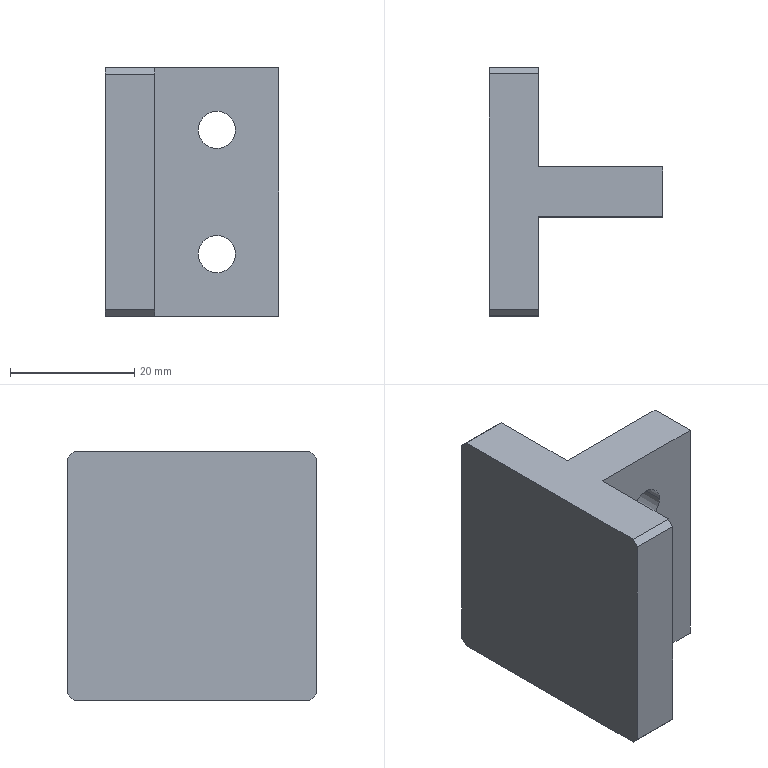Part | SolidWorks | features ICE 2, Chamfer 1, Extrusion 1 | 1 solid | 18 faces | box 28 x 40 x 40 mm | volume 18732 mm3 | plane 14 | cylinder 4 | commonest cylinder face diameters 6 x4
STEP:
#1=CARTESIAN_POINT('',(15.,16.,30.));
#2=VERTEX_POINT('',#1);
#3=CARTESIAN_POINT('',(21.,16.,30.));
#4=VERTEX_POINT('',#3);
#5=CARTESIAN_POINT('',(18.,16.,30.));
#6=DIRECTION('',(0.,-1.,0.));
#7=DIRECTION('',(1.,0.,0.));
#8=AXIS2_PLACEMENT_3D('',#5,#6,#7);
#9=CIRCLE('',#8,3.);
#10=EDGE_CURVE('',#2,#4,#9,.T.);
#11=ORIENTED_EDGE('',*,*,#10,.T.);
#12=CARTESIAN_POINT('',(21.,24.,30.));
#13=VERTEX_POINT('',#12);
#14=CARTESIAN_POINT('',(21.,0.,30.));
#15=DIRECTION('',(0.,1.,0.));
#16=VECTOR('',#15,1000.);
#17=LINE('',#14,#16);
#18=EDGE_CURVE('',#4,#13,#17,.T.);
#19=ORIENTED_EDGE('',*,*,#18,.T.);
#20=CARTESIAN_POINT('',(15.,24.,30.));
#21=VERTEX_POINT('',#20);
#22=CARTESIAN_POINT('',(18.,24.,30.));
#23=DIRECTION('',(0.,1.,0.));
#24=DIRECTION('',(-1.,0.,0.));
#25=AXIS2_PLACEMENT_3D('',#22,#23,#24);
#26=CIRCLE('',#25,3.);
#27=EDGE_CURVE('',#13,#21,#26,.T.);
#28=ORIENTED_EDGE('',*,*,#27,.T.);
#29=CARTESIAN_POINT('',(15.,0.,30.));
#30=DIRECTION('',(0.,1.,0.));
#31=VECTOR('',#30,1000.);
#32=LINE('',#29,#31);
#33=EDGE_CURVE('',#2,#21,#32,.T.);
#34=ORIENTED_EDGE('',*,*,#33,.F.);
#35=EDGE_LOOP('',(#11,#19,#28,#34));
#36=FACE_OUTER_BOUND('',#35,.T.);
#37=CARTESIAN_POINT('',(18.,0.,30.));
#38=DIRECTION('',(0.,1.,0.));
#39=DIRECTION('',(-1.,0.,0.));
#40=AXIS2_PLACEMENT_3D('',#37,#38,#39);
#41=CYLINDRICAL_SURFACE('',#40,3.);
#42=ADVANCED_FACE('',(#36),#41,.F.);
#43=CARTESIAN_POINT('',(15.,16.,10.));
#44=VERTEX_POINT('',#43);
#45=CARTESIAN_POINT('',(21.,16.,10.));
#46=VERTEX_POINT('',#45);
#47=CARTESIAN_POINT('',(18.,16.,10.));
#48=DIRECTION('',(0.,-1.,0.));
#49=DIRECTION('',(1.,0.,0.));
#50=AXIS2_PLACEMENT_3D('',#47,#48,#49);
#51=CIRCLE('',#50,3.);
#52=EDGE_CURVE('',#44,#46,#51,.T.);
#53=ORIENTED_EDGE('',*,*,#52,.T.);
#54=CARTESIAN_POINT('',(21.,24.,10.));
#55=VERTEX_POINT('',#54);
#56=CARTESIAN_POINT('',(21.,0.,10.));
#57=DIRECTION('',(0.,1.,0.));
#58=VECTOR('',#57,1000.);
#59=LINE('',#56,#58);
#60=EDGE_CURVE('',#46,#55,#59,.T.);
#61=ORIENTED_EDGE('',*,*,#60,.T.);
#62=CARTESIAN_POINT('',(15.,24.,10.));
#63=VERTEX_POINT('',#62);
#64=CARTESIAN_POINT('',(18.,24.,10.));
#65=DIRECTION('',(0.,1.,0.));
#66=DIRECTION('',(-1.,0.,0.));
#67=AXIS2_PLACEMENT_3D('',#64,#65,#66);
#68=CIRCLE('',#67,3.);
#69=EDGE_CURVE('',#55,#63,#68,.T.);
#70=ORIENTED_EDGE('',*,*,#69,.T.);
#71=CARTESIAN_POINT('',(15.,0.,10.));
#72=DIRECTION('',(0.,1.,0.));
#73=VECTOR('',#72,1000.);
#74=LINE('',#71,#73);
#75=EDGE_CURVE('',#44,#63,#74,.T.);
#76=ORIENTED_EDGE('',*,*,#75,.F.);
#77=EDGE_LOOP('',(#53,#61,#70,#76));
#78=FACE_OUTER_BOUND('',#77,.T.);
#79=CARTESIAN_POINT('',(18.,0.,10.));
#80=DIRECTION('',(0.,1.,0.));
#81=DIRECTION('',(-1.,0.,0.));
#82=AXIS2_PLACEMENT_3D('',#79,#80,#81);
#83=CYLINDRICAL_SURFACE('',#82,3.);
#84=ADVANCED_FACE('',(#78),#83,.F.);
#85=CARTESIAN_POINT('',(8.,24.,0.));
#86=VERTEX_POINT('',#85);
#87=CARTESIAN_POINT('',(8.,24.,40.));
#88=VERTEX_POINT('',#87);
#89=CARTESIAN_POINT('',(8.,24.,0.));
#90=DIRECTION('',(0.,0.,1.));
#91=VECTOR('',#90,1000.);
#92=LINE('',#89,#91);
#93=EDGE_CURVE('',#86,#88,#92,.T.);
#94=ORIENTED_EDGE('',*,*,#93,.F.);
#95=CARTESIAN_POINT('',(8.,39.,0.));
#96=VERTEX_POINT('',#95);
#97=CARTESIAN_POINT('',(8.,40.,0.));
#98=DIRECTION('',(0.,-1.,0.));
#99=VECTOR('',#98,1000.);
#100=LINE('',#97,#99);
#101=EDGE_CURVE('',#96,#86,#100,.T.);
#102=ORIENTED_EDGE('',*,*,#101,.F.);
#103=CARTESIAN_POINT('',(8.,40.,1.));
#104=VERTEX_POINT('',#103);
#105=CARTESIAN_POINT('',(8.,40.,1.));
#106=DIRECTION('',(0.,0.7071,0.7071));
#107=VECTOR('',#106,1000.);
#108=LINE('',#105,#107);
#109=EDGE_CURVE('',#96,#104,#108,.T.);
#110=ORIENTED_EDGE('',*,*,#109,.T.);
#111=CARTESIAN_POINT('',(8.,40.,39.));
#112=VERTEX_POINT('',#111);
#113=CARTESIAN_POINT('',(8.,40.,0.));
#114=DIRECTION('',(0.,0.,-1.));
#115=VECTOR('',#114,1000.);
#116=LINE('',#113,#115);
#117=EDGE_CURVE('',#112,#104,#116,.T.);
#118=ORIENTED_EDGE('',*,*,#117,.F.);
#119=CARTESIAN_POINT('',(8.,39.,40.));
#120=VERTEX_POINT('',#119);
#121=CARTESIAN_POINT('',(8.,40.,39.));
#122=DIRECTION('',(0.,-0.7071,0.7071));
#123=VECTOR('',#122,1000.);
#124=LINE('',#121,#123);
#125=EDGE_CURVE('',#112,#120,#124,.T.);
#126=ORIENTED_EDGE('',*,*,#125,.T.);
#127=CARTESIAN_POINT('',(8.,40.,40.));
#128=DIRECTION('',(0.,-1.,0.));
#129=VECTOR('',#128,1000.);
#130=LINE('',#127,#129);
#131=EDGE_CURVE('',#120,#88,#130,.T.);
#132=ORIENTED_EDGE('',*,*,#131,.T.);
#133=EDGE_LOOP('',(#94,#102,#110,#118,#126,#132));
#134=FACE_OUTER_BOUND('',#133,.T.);
#135=CARTESIAN_POINT('',(8.,40.,0.));
#136=DIRECTION('',(-1.,0.,0.));
#137=DIRECTION('',(0.,0.,1.));
#138=AXIS2_PLACEMENT_3D('',#135,#136,#137);
#139=PLANE('',#138);
#140=ADVANCED_FACE('',(#134),#139,.F.);
#141=CARTESIAN_POINT('',(0.,39.,40.));
#142=VERTEX_POINT('',#141);
#143=CARTESIAN_POINT('',(0.,1.,40.));
#144=VERTEX_POINT('',#143);
#145=CARTESIAN_POINT('',(0.,40.,40.));
#146=DIRECTION('',(0.,-1.,0.));
#147=VECTOR('',#146,1000.);
#148=LINE('',#145,#147);
#149=EDGE_CURVE('',#142,#144,#148,.T.);
#150=ORIENTED_EDGE('',*,*,#149,.F.);
#151=CARTESIAN_POINT('',(0.,40.,39.));
#152=VERTEX_POINT('',#151);
#153=CARTESIAN_POINT('',(0.,40.,39.));
#154=DIRECTION('',(0.,0.7071,-0.7071));
#155=VECTOR('',#154,1000.);
#156=LINE('',#153,#155);
#157=EDGE_CURVE('',#142,#152,#156,.T.);
#158=ORIENTED_EDGE('',*,*,#157,.T.);
#159=CARTESIAN_POINT('',(0.,40.,1.));
#160=VERTEX_POINT('',#159);
#161=CARTESIAN_POINT('',(0.,40.,0.));
#162=DIRECTION('',(0.,0.,1.));
#163=VECTOR('',#162,1000.);
#164=LINE('',#161,#163);
#165=EDGE_CURVE('',#160,#152,#164,.T.);
#166=ORIENTED_EDGE('',*,*,#165,.F.);
#167=CARTESIAN_POINT('',(0.,39.,0.));
#168=VERTEX_POINT('',#167);
#169=CARTESIAN_POINT('',(0.,40.,1.));
#170=DIRECTION('',(0.,-0.7071,-0.7071));
#171=VECTOR('',#170,1000.);
#172=LINE('',#169,#171);
#173=EDGE_CURVE('',#160,#168,#172,.T.);
#174=ORIENTED_EDGE('',*,*,#173,.T.);
#175=CARTESIAN_POINT('',(0.,1.,0.));
#176=VERTEX_POINT('',#175);
#177=CARTESIAN_POINT('',(0.,40.,0.));
#178=DIRECTION('',(0.,-1.,0.));
#179=VECTOR('',#178,1000.);
#180=LINE('',#177,#179);
#181=EDGE_CURVE('',#168,#176,#180,.T.);
#182=ORIENTED_EDGE('',*,*,#181,.T.);
#183=CARTESIAN_POINT('',(0.,0.,1.));
#184=VERTEX_POINT('',#183);
#185=CARTESIAN_POINT('',(0.,1.,0.));
#186=DIRECTION('',(0.,-0.7071,0.7071));
#187=VECTOR('',#186,1000.);
#188=LINE('',#185,#187);
#189=EDGE_CURVE('',#176,#184,#188,.T.);
#190=ORIENTED_EDGE('',*,*,#189,.T.);
#191=CARTESIAN_POINT('',(0.,0.,39.));
#192=VERTEX_POINT('',#191);
#193=CARTESIAN_POINT('',(0.,0.,0.));
#194=DIRECTION('',(0.,0.,1.));
#195=VECTOR('',#194,1000.);
#196=LINE('',#193,#195);
#197=EDGE_CURVE('',#184,#192,#196,.T.);
#198=ORIENTED_EDGE('',*,*,#197,.T.);
#199=CARTESIAN_POINT('',(0.,1.,40.));
#200=DIRECTION('',(0.,0.7071,0.7071));
#201=VECTOR('',#200,1000.);
#202=LINE('',#199,#201);
#203=EDGE_CURVE('',#192,#144,#202,.T.);
#204=ORIENTED_EDGE('',*,*,#203,.T.);
#205=EDGE_LOOP('',(#150,#158,#166,#174,#182,#190,#198,#204));
#206=FACE_OUTER_BOUND('',#205,.T.);
#207=CARTESIAN_POINT('',(0.,40.,0.));
#208=DIRECTION('',(1.,0.,0.));
#209=DIRECTION('',(0.,0.,-1.));
#210=AXIS2_PLACEMENT_3D('',#207,#208,#209);
#211=PLANE('',#210);
#212=ADVANCED_FACE('',(#206),#211,.F.);
#213=ORIENTED_EDGE('',*,*,#131,.F.);
#214=CARTESIAN_POINT('',(0.,39.,40.));
#215=DIRECTION('',(-1.,0.,0.));
#216=VECTOR('',#215,1000.);
#217=LINE('',#214,#216);
#218=EDGE_CURVE('',#120,#142,#217,.T.);
#219=ORIENTED_EDGE('',*,*,#218,.T.);
#220=ORIENTED_EDGE('',*,*,#149,.T.);
#221=CARTESIAN_POINT('',(8.,1.,40.));
#222=VERTEX_POINT('',#221);
#223=CARTESIAN_POINT('',(0.,1.,40.));
#224=DIRECTION('',(1.,0.,0.));
#225=VECTOR('',#224,1000.);
#226=LINE('',#223,#225);
#227=EDGE_CURVE('',#144,#222,#226,.T.);
#228=ORIENTED_EDGE('',*,*,#227,.T.);
#229=CARTESIAN_POINT('',(8.,16.,40.));
#230=VERTEX_POINT('',#229);
#231=CARTESIAN_POINT('',(8.,40.,40.));
#232=DIRECTION('',(0.,-1.,0.));
#233=VECTOR('',#232,1000.);
#234=LINE('',#231,#233);
#235=EDGE_CURVE('',#230,#222,#234,.T.);
#236=ORIENTED_EDGE('',*,*,#235,.F.);
#237=CARTESIAN_POINT('',(28.,16.,40.));
#238=VERTEX_POINT('',#237);
#239=CARTESIAN_POINT('',(28.,16.,40.));
#240=DIRECTION('',(1.,0.,0.));
#241=VECTOR('',#240,1000.);
#242=LINE('',#239,#241);
#243=EDGE_CURVE('',#230,#238,#242,.T.);
#244=ORIENTED_EDGE('',*,*,#243,.T.);
#245=CARTESIAN_POINT('',(28.,24.,40.));
#246=VERTEX_POINT('',#245);
#247=CARTESIAN_POINT('',(28.,24.,40.));
#248=DIRECTION('',(0.,1.,0.));
#249=VECTOR('',#248,1000.);
#250=LINE('',#247,#249);
#251=EDGE_CURVE('',#238,#246,#250,.T.);
#252=ORIENTED_EDGE('',*,*,#251,.T.);
#253=CARTESIAN_POINT('',(28.,24.,40.));
#254=DIRECTION('',(-1.,0.,0.));
#255=VECTOR('',#254,1000.);
#256=LINE('',#253,#255);
#257=EDGE_CURVE('',#246,#88,#256,.T.);
#258=ORIENTED_EDGE('',*,*,#257,.T.);
#259=EDGE_LOOP('',(#213,#219,#220,#228,#236,#244,#252,#258));
#260=FACE_OUTER_BOUND('',#259,.T.);
#261=CARTESIAN_POINT('',(0.,40.,40.));
#262=DIRECTION('',(0.,0.,-1.));
#263=DIRECTION('',(-1.,0.,0.));
#264=AXIS2_PLACEMENT_3D('',#261,#262,#263);
#265=PLANE('',#264);
#266=ADVANCED_FACE('',(#260),#265,.F.);
#267=CARTESIAN_POINT('',(8.,16.,0.));
#268=VERTEX_POINT('',#267);
#269=CARTESIAN_POINT('',(8.,1.,0.));
#270=VERTEX_POINT('',#269);
#271=CARTESIAN_POINT('',(8.,40.,0.));
#272=DIRECTION('',(0.,-1.,0.));
#273=VECTOR('',#272,1000.);
#274=LINE('',#271,#273);
#275=EDGE_CURVE('',#268,#270,#274,.T.);
#276=ORIENTED_EDGE('',*,*,#275,.F.);
#277=CARTESIAN_POINT('',(8.,16.,0.));
#278=DIRECTION('',(0.,0.,1.));
#279=VECTOR('',#278,1000.);
#280=LINE('',#277,#279);
#281=EDGE_CURVE('',#268,#230,#280,.T.);
#282=ORIENTED_EDGE('',*,*,#281,.T.);
#283=ORIENTED_EDGE('',*,*,#235,.T.);
#284=CARTESIAN_POINT('',(8.,0.,39.));
#285=VERTEX_POINT('',#284);
#286=CARTESIAN_POINT('',(8.,1.,40.));
#287=DIRECTION('',(0.,-0.7071,-0.7071));
#288=VECTOR('',#287,1000.);
#289=LINE('',#286,#288);
#290=EDGE_CURVE('',#222,#285,#289,.T.);
#291=ORIENTED_EDGE('',*,*,#290,.T.);
#292=CARTESIAN_POINT('',(8.,0.,1.));
#293=VERTEX_POINT('',#292);
#294=CARTESIAN_POINT('',(8.,0.,0.));
#295=DIRECTION('',(0.,0.,-1.));
#296=VECTOR('',#295,1000.);
#297=LINE('',#294,#296);
#298=EDGE_CURVE('',#285,#293,#297,.T.);
#299=ORIENTED_EDGE('',*,*,#298,.T.);
#300=CARTESIAN_POINT('',(8.,1.,0.));
#301=DIRECTION('',(0.,0.7071,-0.7071));
#302=VECTOR('',#301,1000.);
#303=LINE('',#300,#302);
#304=EDGE_CURVE('',#293,#270,#303,.T.);
#305=ORIENTED_EDGE('',*,*,#304,.T.);
#306=EDGE_LOOP('',(#276,#282,#283,#291,#299,#305));
#307=FACE_OUTER_BOUND('',#306,.T.);
#308=CARTESIAN_POINT('',(8.,40.,0.));
#309=DIRECTION('',(-1.,0.,0.));
#310=DIRECTION('',(0.,0.,1.));
#311=AXIS2_PLACEMENT_3D('',#308,#309,#310);
#312=PLANE('',#311);
#313=ADVANCED_FACE('',(#307),#312,.F.);
#314=ORIENTED_EDGE('',*,*,#181,.F.);
#315=CARTESIAN_POINT('',(8.,39.,0.));
#316=DIRECTION('',(1.,0.,0.));
#317=VECTOR('',#316,1000.);
#318=LINE('',#315,#317);
#319=EDGE_CURVE('',#168,#96,#318,.T.);
#320=ORIENTED_EDGE('',*,*,#319,.T.);
#321=ORIENTED_EDGE('',*,*,#101,.T.);
#322=CARTESIAN_POINT('',(28.,24.,0.));
#323=VERTEX_POINT('',#322);
#324=CARTESIAN_POINT('',(28.,24.,0.));
#325=DIRECTION('',(-1.,0.,0.));
#326=VECTOR('',#325,1000.);
#327=LINE('',#324,#326);
#328=EDGE_CURVE('',#323,#86,#327,.T.);
#329=ORIENTED_EDGE('',*,*,#328,.F.);
#330=CARTESIAN_POINT('',(28.,16.,0.));
#331=VERTEX_POINT('',#330);
#332=CARTESIAN_POINT('',(28.,24.,0.));
#333=DIRECTION('',(0.,1.,0.));
#334=VECTOR('',#333,1000.);
#335=LINE('',#332,#334);
#336=EDGE_CURVE('',#331,#323,#335,.T.);
#337=ORIENTED_EDGE('',*,*,#336,.F.);
#338=CARTESIAN_POINT('',(28.,16.,0.));
#339=DIRECTION('',(1.,0.,0.));
#340=VECTOR('',#339,1000.);
#341=LINE('',#338,#340);
#342=EDGE_CURVE('',#268,#331,#341,.T.);
#343=ORIENTED_EDGE('',*,*,#342,.F.);
#344=ORIENTED_EDGE('',*,*,#275,.T.);
#345=CARTESIAN_POINT('',(0.,1.,0.));
#346=DIRECTION('',(-1.,0.,0.));
#347=VECTOR('',#346,1000.);
#348=LINE('',#345,#347);
#349=EDGE_CURVE('',#270,#176,#348,.T.);
#350=ORIENTED_EDGE('',*,*,#349,.T.);
#351=EDGE_LOOP('',(#314,#320,#321,#329,#337,#343,#344,#350));
#352=FACE_OUTER_BOUND('',#351,.T.);
#353=CARTESIAN_POINT('',(0.,40.,0.));
#354=DIRECTION('',(0.,0.,1.));
#355=DIRECTION('',(1.,0.,0.));
#356=AXIS2_PLACEMENT_3D('',#353,#354,#355);
#357=PLANE('',#356);
#358=ADVANCED_FACE('',(#352),#357,.F.);
#359=ORIENTED_EDGE('',*,*,#165,.T.);
#360=CARTESIAN_POINT('',(8.,40.,39.));
#361=DIRECTION('',(1.,0.,0.));
#362=VECTOR('',#361,1000.);
#363=LINE('',#360,#362);
#364=EDGE_CURVE('',#152,#112,#363,.T.);
#365=ORIENTED_EDGE('',*,*,#364,.T.);
#366=ORIENTED_EDGE('',*,*,#117,.T.);
#367=CARTESIAN_POINT('',(0.,40.,1.));
#368=DIRECTION('',(-1.,0.,0.));
#369=VECTOR('',#368,1000.);
#370=LINE('',#367,#369);
#371=EDGE_CURVE('',#104,#160,#370,.T.);
#372=ORIENTED_EDGE('',*,*,#371,.T.);
#373=EDGE_LOOP('',(#359,#365,#366,#372));
#374=FACE_OUTER_BOUND('',#373,.T.);
#375=CARTESIAN_POINT('',(0.,40.,0.));
#376=DIRECTION('',(0.,1.,0.));
#377=DIRECTION('',(0.,0.,1.));
#378=AXIS2_PLACEMENT_3D('',#375,#376,#377);
#379=PLANE('',#378);
#380=ADVANCED_FACE('',(#374),#379,.T.);
#381=ORIENTED_EDGE('',*,*,#298,.F.);
#382=CARTESIAN_POINT('',(0.,0.,39.));
#383=DIRECTION('',(-1.,0.,0.));
#384=VECTOR('',#383,1000.);
#385=LINE('',#382,#384);
#386=EDGE_CURVE('',#285,#192,#385,.T.);
#387=ORIENTED_EDGE('',*,*,#386,.T.);
#388=ORIENTED_EDGE('',*,*,#197,.F.);
#389=CARTESIAN_POINT('',(0.,0.,1.));
#390=DIRECTION('',(1.,0.,0.));
#391=VECTOR('',#390,1000.);
#392=LINE('',#389,#391);
#393=EDGE_CURVE('',#184,#293,#392,.T.);
#394=ORIENTED_EDGE('',*,*,#393,.T.);
#395=EDGE_LOOP('',(#381,#387,#388,#394));
#396=FACE_OUTER_BOUND('',#395,.T.);
#397=CARTESIAN_POINT('',(0.,0.,0.));
#398=DIRECTION('',(0.,1.,0.));
#399=DIRECTION('',(0.,0.,1.));
#400=AXIS2_PLACEMENT_3D('',#397,#398,#399);
#401=PLANE('',#400);
#402=ADVANCED_FACE('',(#396),#401,.F.);
#403=ORIENTED_EDGE('',*,*,#157,.F.);
#404=ORIENTED_EDGE('',*,*,#218,.F.);
#405=ORIENTED_EDGE('',*,*,#125,.F.);
#406=ORIENTED_EDGE('',*,*,#364,.F.);
#407=EDGE_LOOP('',(#403,#404,#405,#406));
#408=FACE_OUTER_BOUND('',#407,.T.);
#409=CARTESIAN_POINT('',(0.,40.,39.));
#410=DIRECTION('',(0.,0.7071,0.7071));
#411=DIRECTION('',(-1.,0.,0.));
#412=AXIS2_PLACEMENT_3D('',#409,#410,#411);
#413=PLANE('',#412);
#414=ADVANCED_FACE('',(#408),#413,.T.);
#415=ORIENTED_EDGE('',*,*,#203,.F.);
#416=ORIENTED_EDGE('',*,*,#386,.F.);
#417=ORIENTED_EDGE('',*,*,#290,.F.);
#418=ORIENTED_EDGE('',*,*,#227,.F.);
#419=EDGE_LOOP('',(#415,#416,#417,#418));
#420=FACE_OUTER_BOUND('',#419,.T.);
#421=CARTESIAN_POINT('',(0.,1.,40.));
#422=DIRECTION('',(0.,0.7071,-0.7071));
#423=DIRECTION('',(1.,0.,0.));
#424=AXIS2_PLACEMENT_3D('',#421,#422,#423);
#425=PLANE('',#424);
#426=ADVANCED_FACE('',(#420),#425,.F.);
#427=ORIENTED_EDGE('',*,*,#109,.F.);
#428=ORIENTED_EDGE('',*,*,#319,.F.);
#429=ORIENTED_EDGE('',*,*,#173,.F.);
#430=ORIENTED_EDGE('',*,*,#371,.F.);
#431=EDGE_LOOP('',(#427,#428,#429,#430));
#432=FACE_OUTER_BOUND('',#431,.T.);
#433=CARTESIAN_POINT('',(0.,40.,1.));
#434=DIRECTION('',(0.,0.7071,-0.7071));
#435=DIRECTION('',(1.,0.,0.));
#436=AXIS2_PLACEMENT_3D('',#433,#434,#435);
#437=PLANE('',#436);
#438=ADVANCED_FACE('',(#432),#437,.T.);
#439=ORIENTED_EDGE('',*,*,#304,.F.);
#440=ORIENTED_EDGE('',*,*,#393,.F.);
#441=ORIENTED_EDGE('',*,*,#189,.F.);
#442=ORIENTED_EDGE('',*,*,#349,.F.);
#443=EDGE_LOOP('',(#439,#440,#441,#442));
#444=FACE_OUTER_BOUND('',#443,.T.);
#445=CARTESIAN_POINT('',(0.,1.,0.));
#446=DIRECTION('',(0.,0.7071,0.7071));
#447=DIRECTION('',(-1.,0.,0.));
#448=AXIS2_PLACEMENT_3D('',#445,#446,#447);
#449=PLANE('',#448);
#450=ADVANCED_FACE('',(#444),#449,.F.);
#451=ORIENTED_EDGE('',*,*,#251,.F.);
#452=CARTESIAN_POINT('',(28.,16.,0.));
#453=DIRECTION('',(0.,0.,1.));
#454=VECTOR('',#453,1000.);
#455=LINE('',#452,#454);
#456=EDGE_CURVE('',#331,#238,#455,.T.);
#457=ORIENTED_EDGE('',*,*,#456,.F.);
#458=ORIENTED_EDGE('',*,*,#336,.T.);
#459=CARTESIAN_POINT('',(28.,24.,0.));
#460=DIRECTION('',(0.,0.,1.));
#461=VECTOR('',#460,1000.);
#462=LINE('',#459,#461);
#463=EDGE_CURVE('',#323,#246,#462,.T.);
#464=ORIENTED_EDGE('',*,*,#463,.T.);
#465=EDGE_LOOP('',(#451,#457,#458,#464));
#466=FACE_OUTER_BOUND('',#465,.T.);
#467=CARTESIAN_POINT('',(28.,24.,0.));
#468=DIRECTION('',(1.,0.,0.));
#469=DIRECTION('',(0.,1.,0.));
#470=AXIS2_PLACEMENT_3D('',#467,#468,#469);
#471=PLANE('',#470);
#472=ADVANCED_FACE('',(#466),#471,.T.);
#473=ORIENTED_EDGE('',*,*,#10,.F.);
#474=CARTESIAN_POINT('',(18.,16.,30.));
#475=DIRECTION('',(0.,-1.,0.));
#476=DIRECTION('',(1.,0.,0.));
#477=AXIS2_PLACEMENT_3D('',#474,#475,#476);
#478=CIRCLE('',#477,3.);
#479=EDGE_CURVE('',#4,#2,#478,.T.);
#480=ORIENTED_EDGE('',*,*,#479,.F.);
#481=EDGE_LOOP('',(#473,#480));
#482=FACE_BOUND('',#481,.T.);
#483=ORIENTED_EDGE('',*,*,#52,.F.);
#484=CARTESIAN_POINT('',(18.,16.,10.));
#485=DIRECTION('',(0.,-1.,0.));
#486=DIRECTION('',(1.,0.,0.));
#487=AXIS2_PLACEMENT_3D('',#484,#485,#486);
#488=CIRCLE('',#487,3.);
#489=EDGE_CURVE('',#46,#44,#488,.T.);
#490=ORIENTED_EDGE('',*,*,#489,.F.);
#491=EDGE_LOOP('',(#483,#490));
#492=FACE_BOUND('',#491,.T.);
#493=ORIENTED_EDGE('',*,*,#243,.F.);
#494=ORIENTED_EDGE('',*,*,#281,.F.);
#495=ORIENTED_EDGE('',*,*,#342,.T.);
#496=ORIENTED_EDGE('',*,*,#456,.T.);
#497=EDGE_LOOP('',(#493,#494,#495,#496));
#498=FACE_OUTER_BOUND('',#497,.T.);
#499=CARTESIAN_POINT('',(28.,16.,0.));
#500=DIRECTION('',(0.,-1.,0.));
#501=DIRECTION('',(1.,0.,0.));
#502=AXIS2_PLACEMENT_3D('',#499,#500,#501);
#503=PLANE('',#502);
#504=ADVANCED_FACE('',(#482,#492,#498),#503,.T.);
#505=CARTESIAN_POINT('',(18.,24.,30.));
#506=DIRECTION('',(0.,1.,0.));
#507=DIRECTION('',(-1.,0.,0.));
#508=AXIS2_PLACEMENT_3D('',#505,#506,#507);
#509=CIRCLE('',#508,3.);
#510=EDGE_CURVE('',#21,#13,#509,.T.);
#511=ORIENTED_EDGE('',*,*,#510,.F.);
#512=ORIENTED_EDGE('',*,*,#27,.F.);
#513=EDGE_LOOP('',(#511,#512));
#514=FACE_BOUND('',#513,.T.);
#515=CARTESIAN_POINT('',(18.,24.,10.));
#516=DIRECTION('',(0.,1.,0.));
#517=DIRECTION('',(-1.,0.,0.));
#518=AXIS2_PLACEMENT_3D('',#515,#516,#517);
#519=CIRCLE('',#518,3.);
#520=EDGE_CURVE('',#63,#55,#519,.T.);
#521=ORIENTED_EDGE('',*,*,#520,.F.);
#522=ORIENTED_EDGE('',*,*,#69,.F.);
#523=EDGE_LOOP('',(#521,#522));
#524=FACE_BOUND('',#523,.T.);
#525=ORIENTED_EDGE('',*,*,#257,.F.);
#526=ORIENTED_EDGE('',*,*,#463,.F.);
#527=ORIENTED_EDGE('',*,*,#328,.T.);
#528=ORIENTED_EDGE('',*,*,#93,.T.);
#529=EDGE_LOOP('',(#525,#526,#527,#528));
#530=FACE_OUTER_BOUND('',#529,.T.);
#531=CARTESIAN_POINT('',(28.,24.,0.));
#532=DIRECTION('',(0.,1.,0.));
#533=DIRECTION('',(-1.,0.,0.));
#534=AXIS2_PLACEMENT_3D('',#531,#532,#533);
#535=PLANE('',#534);
#536=ADVANCED_FACE('',(#514,#524,#530),#535,.T.);
#537=ORIENTED_EDGE('',*,*,#60,.F.);
#538=ORIENTED_EDGE('',*,*,#489,.T.);
#539=ORIENTED_EDGE('',*,*,#75,.T.);
#540=ORIENTED_EDGE('',*,*,#520,.T.);
#541=EDGE_LOOP('',(#537,#538,#539,#540));
#542=FACE_OUTER_BOUND('',#541,.T.);
#543=CARTESIAN_POINT('',(18.,0.,10.));
#544=DIRECTION('',(0.,1.,0.));
#545=DIRECTION('',(-1.,0.,0.));
#546=AXIS2_PLACEMENT_3D('',#543,#544,#545);
#547=CYLINDRICAL_SURFACE('',#546,3.);
#548=ADVANCED_FACE('',(#542),#547,.F.);
#549=ORIENTED_EDGE('',*,*,#18,.F.);
#550=ORIENTED_EDGE('',*,*,#479,.T.);
#551=ORIENTED_EDGE('',*,*,#33,.T.);
#552=ORIENTED_EDGE('',*,*,#510,.T.);
#553=EDGE_LOOP('',(#549,#550,#551,#552));
#554=FACE_OUTER_BOUND('',#553,.T.);
#555=CARTESIAN_POINT('',(18.,0.,30.));
#556=DIRECTION('',(0.,1.,0.));
#557=DIRECTION('',(-1.,0.,0.));
#558=AXIS2_PLACEMENT_3D('',#555,#556,#557);
#559=CYLINDRICAL_SURFACE('',#558,3.);
#560=ADVANCED_FACE('',(#554),#559,.F.);
#561=CLOSED_SHELL('',(#42,#84,#140,#212,#266,#313,#358,#380,#402,#414,#426,#438,#450,#472,#504,#536,#548,#560));
#562=MANIFOLD_SOLID_BREP('',#561);
#563=CARTESIAN_POINT('',(0.,0.,0.));
#564=DIRECTION('',(0.,0.,1.));
#565=DIRECTION('',(1.,0.,0.));
#566=AXIS2_PLACEMENT_3D('',#563,#564,#565);
#567=(LENGTH_UNIT()NAMED_UNIT(*)SI_UNIT(.MILLI.,.METRE.));
#568=UNCERTAINTY_MEASURE_WITH_UNIT(LENGTH_MEASURE(0.00001),#567,'','');
#569=(NAMED_UNIT(*)PLANE_ANGLE_UNIT()SI_UNIT($,.RADIAN.));
#570=(NAMED_UNIT(*)SI_UNIT($,.STERADIAN.)SOLID_ANGLE_UNIT());
#571=(GEOMETRIC_REPRESENTATION_CONTEXT(3)GLOBAL_UNCERTAINTY_ASSIGNED_CONTEXT((#568))GLOBAL_UNIT_ASSIGNED_CONTEXT((#567,#569,#570))REPRESENTATION_CONTEXT('',''));
#572=ADVANCED_BREP_SHAPE_REPRESENTATION('',(#562,#566),#571);